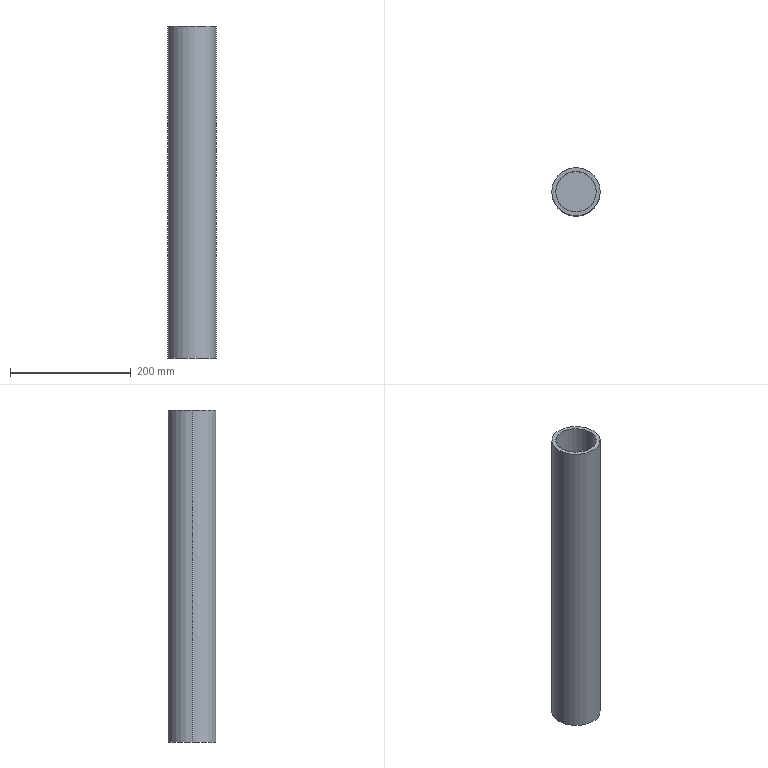Part | SolidWorks | features Extrusion 1, ICE 1 | 1 solid | 7 faces | box 80 x 80 x 550 mm | volume 2447293 mm3 | cylinder 4 | plane 3 | commonest cylinder face diameters 67 x2 80 x2
STEP:
#1=CARTESIAN_POINT('',(-33.5,0.,460.));
#2=VERTEX_POINT('',#1);
#3=CARTESIAN_POINT('',(33.5,0.,460.));
#4=VERTEX_POINT('',#3);
#5=CARTESIAN_POINT('',(0.,0.,460.));
#6=DIRECTION('',(0.,0.,1.));
#7=DIRECTION('',(1.,0.,0.));
#8=AXIS2_PLACEMENT_3D('',#5,#6,#7);
#9=CIRCLE('',#8,33.5);
#10=EDGE_CURVE('',#2,#4,#9,.T.);
#11=ORIENTED_EDGE('',*,*,#10,.F.);
#12=CARTESIAN_POINT('',(-33.5,0.,550.));
#13=VERTEX_POINT('',#12);
#14=CARTESIAN_POINT('',(-33.5,0.,460.));
#15=DIRECTION('',(0.,0.,1.));
#16=VECTOR('',#15,1000.);
#17=LINE('',#14,#16);
#18=EDGE_CURVE('',#2,#13,#17,.T.);
#19=ORIENTED_EDGE('',*,*,#18,.T.);
#20=CARTESIAN_POINT('',(33.5,0.,550.));
#21=VERTEX_POINT('',#20);
#22=CARTESIAN_POINT('',(0.,0.,550.));
#23=DIRECTION('',(0.,0.,1.));
#24=DIRECTION('',(1.,0.,0.));
#25=AXIS2_PLACEMENT_3D('',#22,#23,#24);
#26=CIRCLE('',#25,33.5);
#27=EDGE_CURVE('',#13,#21,#26,.T.);
#28=ORIENTED_EDGE('',*,*,#27,.T.);
#29=CARTESIAN_POINT('',(33.5,0.,460.));
#30=DIRECTION('',(0.,0.,1.));
#31=VECTOR('',#30,1000.);
#32=LINE('',#29,#31);
#33=EDGE_CURVE('',#4,#21,#32,.T.);
#34=ORIENTED_EDGE('',*,*,#33,.F.);
#35=EDGE_LOOP('',(#11,#19,#28,#34));
#36=FACE_OUTER_BOUND('',#35,.T.);
#37=CARTESIAN_POINT('',(0.,0.,460.));
#38=DIRECTION('',(0.,0.,1.));
#39=DIRECTION('',(1.,0.,0.));
#40=AXIS2_PLACEMENT_3D('',#37,#38,#39);
#41=CYLINDRICAL_SURFACE('',#40,33.5);
#42=ADVANCED_FACE('',(#36),#41,.F.);
#43=CARTESIAN_POINT('',(40.,0.,550.));
#44=VERTEX_POINT('',#43);
#45=CARTESIAN_POINT('',(-40.,0.,550.));
#46=VERTEX_POINT('',#45);
#47=CARTESIAN_POINT('',(0.,0.,550.));
#48=DIRECTION('',(0.,0.,1.));
#49=DIRECTION('',(1.,0.,0.));
#50=AXIS2_PLACEMENT_3D('',#47,#48,#49);
#51=CIRCLE('',#50,40.);
#52=EDGE_CURVE('',#44,#46,#51,.T.);
#53=ORIENTED_EDGE('',*,*,#52,.F.);
#54=CARTESIAN_POINT('',(40.,0.,0.));
#55=VERTEX_POINT('',#54);
#56=CARTESIAN_POINT('',(40.,0.,550.));
#57=DIRECTION('',(0.,0.,-1.));
#58=VECTOR('',#57,1000.);
#59=LINE('',#56,#58);
#60=EDGE_CURVE('',#44,#55,#59,.T.);
#61=ORIENTED_EDGE('',*,*,#60,.T.);
#62=CARTESIAN_POINT('',(-40.,0.,0.));
#63=VERTEX_POINT('',#62);
#64=CARTESIAN_POINT('',(0.,0.,0.));
#65=DIRECTION('',(0.,0.,1.));
#66=DIRECTION('',(1.,0.,0.));
#67=AXIS2_PLACEMENT_3D('',#64,#65,#66);
#68=CIRCLE('',#67,40.);
#69=EDGE_CURVE('',#55,#63,#68,.T.);
#70=ORIENTED_EDGE('',*,*,#69,.T.);
#71=CARTESIAN_POINT('',(-40.,0.,550.));
#72=DIRECTION('',(0.,0.,-1.));
#73=VECTOR('',#72,1000.);
#74=LINE('',#71,#73);
#75=EDGE_CURVE('',#46,#63,#74,.T.);
#76=ORIENTED_EDGE('',*,*,#75,.F.);
#77=EDGE_LOOP('',(#53,#61,#70,#76));
#78=FACE_OUTER_BOUND('',#77,.T.);
#79=CARTESIAN_POINT('',(0.,0.,550.));
#80=DIRECTION('',(0.,0.,-1.));
#81=DIRECTION('',(-1.,0.,0.));
#82=AXIS2_PLACEMENT_3D('',#79,#80,#81);
#83=CYLINDRICAL_SURFACE('',#82,40.);
#84=ADVANCED_FACE('',(#78),#83,.T.);
#85=ORIENTED_EDGE('',*,*,#60,.F.);
#86=CARTESIAN_POINT('',(0.,0.,550.));
#87=DIRECTION('',(0.,0.,1.));
#88=DIRECTION('',(1.,0.,0.));
#89=AXIS2_PLACEMENT_3D('',#86,#87,#88);
#90=CIRCLE('',#89,40.);
#91=EDGE_CURVE('',#46,#44,#90,.T.);
#92=ORIENTED_EDGE('',*,*,#91,.F.);
#93=ORIENTED_EDGE('',*,*,#75,.T.);
#94=CARTESIAN_POINT('',(0.,0.,0.));
#95=DIRECTION('',(0.,0.,1.));
#96=DIRECTION('',(1.,0.,0.));
#97=AXIS2_PLACEMENT_3D('',#94,#95,#96);
#98=CIRCLE('',#97,40.);
#99=EDGE_CURVE('',#63,#55,#98,.T.);
#100=ORIENTED_EDGE('',*,*,#99,.T.);
#101=EDGE_LOOP('',(#85,#92,#93,#100));
#102=FACE_OUTER_BOUND('',#101,.T.);
#103=CARTESIAN_POINT('',(0.,0.,550.));
#104=DIRECTION('',(0.,0.,-1.));
#105=DIRECTION('',(-1.,0.,0.));
#106=AXIS2_PLACEMENT_3D('',#103,#104,#105);
#107=CYLINDRICAL_SURFACE('',#106,40.);
#108=ADVANCED_FACE('',(#102),#107,.T.);
#109=CARTESIAN_POINT('',(0.,0.,550.));
#110=DIRECTION('',(0.,0.,1.));
#111=DIRECTION('',(1.,0.,0.));
#112=AXIS2_PLACEMENT_3D('',#109,#110,#111);
#113=CIRCLE('',#112,33.5);
#114=EDGE_CURVE('',#21,#13,#113,.T.);
#115=ORIENTED_EDGE('',*,*,#114,.F.);
#116=ORIENTED_EDGE('',*,*,#27,.F.);
#117=EDGE_LOOP('',(#115,#116));
#118=FACE_BOUND('',#117,.T.);
#119=ORIENTED_EDGE('',*,*,#91,.T.);
#120=ORIENTED_EDGE('',*,*,#52,.T.);
#121=EDGE_LOOP('',(#119,#120));
#122=FACE_OUTER_BOUND('',#121,.T.);
#123=CARTESIAN_POINT('',(0.,0.,550.));
#124=DIRECTION('',(0.,0.,1.));
#125=DIRECTION('',(1.,0.,0.));
#126=AXIS2_PLACEMENT_3D('',#123,#124,#125);
#127=PLANE('',#126);
#128=ADVANCED_FACE('',(#118,#122),#127,.T.);
#129=ORIENTED_EDGE('',*,*,#99,.F.);
#130=ORIENTED_EDGE('',*,*,#69,.F.);
#131=EDGE_LOOP('',(#129,#130));
#132=FACE_OUTER_BOUND('',#131,.T.);
#133=CARTESIAN_POINT('',(0.,0.,0.));
#134=DIRECTION('',(0.,0.,1.));
#135=DIRECTION('',(1.,0.,0.));
#136=AXIS2_PLACEMENT_3D('',#133,#134,#135);
#137=PLANE('',#136);
#138=ADVANCED_FACE('',(#132),#137,.F.);
#139=ORIENTED_EDGE('',*,*,#18,.F.);
#140=CARTESIAN_POINT('',(0.,0.,460.));
#141=DIRECTION('',(0.,0.,1.));
#142=DIRECTION('',(1.,0.,0.));
#143=AXIS2_PLACEMENT_3D('',#140,#141,#142);
#144=CIRCLE('',#143,33.5);
#145=EDGE_CURVE('',#4,#2,#144,.T.);
#146=ORIENTED_EDGE('',*,*,#145,.F.);
#147=ORIENTED_EDGE('',*,*,#33,.T.);
#148=ORIENTED_EDGE('',*,*,#114,.T.);
#149=EDGE_LOOP('',(#139,#146,#147,#148));
#150=FACE_OUTER_BOUND('',#149,.T.);
#151=CARTESIAN_POINT('',(0.,0.,460.));
#152=DIRECTION('',(0.,0.,1.));
#153=DIRECTION('',(1.,0.,0.));
#154=AXIS2_PLACEMENT_3D('',#151,#152,#153);
#155=CYLINDRICAL_SURFACE('',#154,33.5);
#156=ADVANCED_FACE('',(#150),#155,.F.);
#157=ORIENTED_EDGE('',*,*,#145,.T.);
#158=ORIENTED_EDGE('',*,*,#10,.T.);
#159=EDGE_LOOP('',(#157,#158));
#160=FACE_OUTER_BOUND('',#159,.T.);
#161=CARTESIAN_POINT('',(0.,0.,460.));
#162=DIRECTION('',(0.,0.,1.));
#163=DIRECTION('',(1.,0.,0.));
#164=AXIS2_PLACEMENT_3D('',#161,#162,#163);
#165=PLANE('',#164);
#166=ADVANCED_FACE('',(#160),#165,.T.);
#167=CLOSED_SHELL('',(#42,#84,#108,#128,#138,#156,#166));
#168=MANIFOLD_SOLID_BREP('',#167);
#169=CARTESIAN_POINT('',(0.,0.,0.));
#170=DIRECTION('',(0.,0.,1.));
#171=DIRECTION('',(1.,0.,0.));
#172=AXIS2_PLACEMENT_3D('',#169,#170,#171);
#173=(LENGTH_UNIT()NAMED_UNIT(*)SI_UNIT(.MILLI.,.METRE.));
#174=UNCERTAINTY_MEASURE_WITH_UNIT(LENGTH_MEASURE(0.00001),#173,'','');
#175=(NAMED_UNIT(*)PLANE_ANGLE_UNIT()SI_UNIT($,.RADIAN.));
#176=(NAMED_UNIT(*)SI_UNIT($,.STERADIAN.)SOLID_ANGLE_UNIT());
#177=(GEOMETRIC_REPRESENTATION_CONTEXT(3)GLOBAL_UNCERTAINTY_ASSIGNED_CONTEXT((#174))GLOBAL_UNIT_ASSIGNED_CONTEXT((#173,#175,#176))REPRESENTATION_CONTEXT('',''));
#178=ADVANCED_BREP_SHAPE_REPRESENTATION('',(#168,#172),#177);